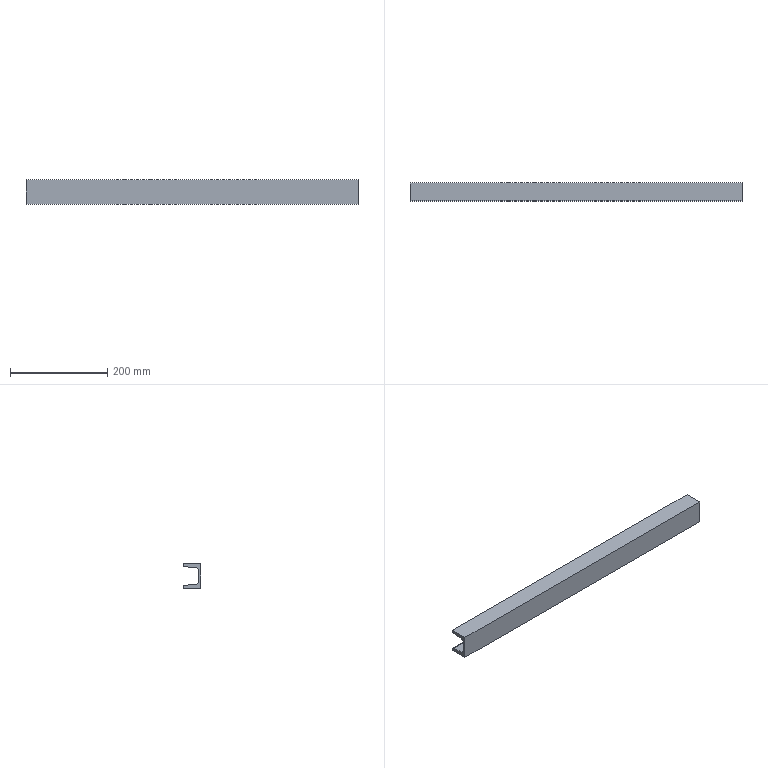Part | SolidWorks | features WeldMemberFeat 1, WeldmentFeature 1 | 1 solid | 14 faces | box 684 x 37 x 50 mm | volume 473534 mm3 | plane 10 | cylinder 4 | commonest cylinder face diameters 7 x2 14 x2
STEP:
#1=CARTESIAN_POINT('',(-342.,33.866,44.379));
#2=VERTEX_POINT('',#1);
#3=CARTESIAN_POINT('',(-342.,37.,47.859));
#4=VERTEX_POINT('',#3);
#5=CARTESIAN_POINT('',(-342.,33.5,47.859));
#6=DIRECTION('',(1.,0.,0.));
#7=DIRECTION('',(0.,1.,0.));
#8=AXIS2_PLACEMENT_3D('',#5,#6,#7);
#9=CIRCLE('',#8,3.5);
#10=EDGE_CURVE('',#2,#4,#9,.T.);
#11=ORIENTED_EDGE('',*,*,#10,.T.);
#12=CARTESIAN_POINT('',(342.,37.,47.859));
#13=VERTEX_POINT('',#12);
#14=CARTESIAN_POINT('',(342.,37.,47.859));
#15=DIRECTION('',(-1.,0.,0.));
#16=VECTOR('',#15,1000.);
#17=LINE('',#14,#16);
#18=EDGE_CURVE('',#13,#4,#17,.T.);
#19=ORIENTED_EDGE('',*,*,#18,.F.);
#20=CARTESIAN_POINT('',(342.,33.866,44.379));
#21=VERTEX_POINT('',#20);
#22=CARTESIAN_POINT('',(342.,33.5,47.859));
#23=DIRECTION('',(1.,0.,0.));
#24=DIRECTION('',(0.,1.,0.));
#25=AXIS2_PLACEMENT_3D('',#22,#23,#24);
#26=CIRCLE('',#25,3.5);
#27=EDGE_CURVE('',#21,#13,#26,.T.);
#28=ORIENTED_EDGE('',*,*,#27,.F.);
#29=CARTESIAN_POINT('',(342.,33.866,44.379));
#30=DIRECTION('',(-1.,0.,0.));
#31=VECTOR('',#30,1000.);
#32=LINE('',#29,#31);
#33=EDGE_CURVE('',#21,#2,#32,.T.);
#34=ORIENTED_EDGE('',*,*,#33,.T.);
#35=EDGE_LOOP('',(#11,#19,#28,#34));
#36=FACE_OUTER_BOUND('',#35,.T.);
#37=CARTESIAN_POINT('',(342.,33.5,47.859));
#38=DIRECTION('',(-1.,0.,0.));
#39=DIRECTION('',(0.,-1.,0.));
#40=AXIS2_PLACEMENT_3D('',#37,#38,#39);
#41=CYLINDRICAL_SURFACE('',#40,3.5);
#42=ADVANCED_FACE('',(#36),#41,.T.);
#43=CARTESIAN_POINT('',(-342.,37.,50.));
#44=VERTEX_POINT('',#43);
#45=CARTESIAN_POINT('',(-342.,37.,50.));
#46=DIRECTION('',(0.,0.,1.));
#47=VECTOR('',#46,1000.);
#48=LINE('',#45,#47);
#49=EDGE_CURVE('',#4,#44,#48,.T.);
#50=ORIENTED_EDGE('',*,*,#49,.T.);
#51=CARTESIAN_POINT('',(342.,37.,50.));
#52=VERTEX_POINT('',#51);
#53=CARTESIAN_POINT('',(342.,37.,50.));
#54=DIRECTION('',(-1.,0.,0.));
#55=VECTOR('',#54,1000.);
#56=LINE('',#53,#55);
#57=EDGE_CURVE('',#52,#44,#56,.T.);
#58=ORIENTED_EDGE('',*,*,#57,.F.);
#59=CARTESIAN_POINT('',(342.,37.,50.));
#60=DIRECTION('',(0.,0.,1.));
#61=VECTOR('',#60,1000.);
#62=LINE('',#59,#61);
#63=EDGE_CURVE('',#13,#52,#62,.T.);
#64=ORIENTED_EDGE('',*,*,#63,.F.);
#65=ORIENTED_EDGE('',*,*,#18,.T.);
#66=EDGE_LOOP('',(#50,#58,#64,#65));
#67=FACE_OUTER_BOUND('',#66,.T.);
#68=CARTESIAN_POINT('',(342.,37.,50.));
#69=DIRECTION('',(0.,-1.,0.));
#70=DIRECTION('',(1.,0.,0.));
#71=AXIS2_PLACEMENT_3D('',#68,#69,#70);
#72=PLANE('',#71);
#73=ADVANCED_FACE('',(#67),#72,.F.);
#74=CARTESIAN_POINT('',(-342.,0.,50.));
#75=VERTEX_POINT('',#74);
#76=CARTESIAN_POINT('',(-342.,37.,50.));
#77=DIRECTION('',(0.,-1.,0.));
#78=VECTOR('',#77,1000.);
#79=LINE('',#76,#78);
#80=EDGE_CURVE('',#44,#75,#79,.T.);
#81=ORIENTED_EDGE('',*,*,#80,.T.);
#82=CARTESIAN_POINT('',(342.,0.,50.));
#83=VERTEX_POINT('',#82);
#84=CARTESIAN_POINT('',(342.,0.,50.));
#85=DIRECTION('',(-1.,0.,0.));
#86=VECTOR('',#85,1000.);
#87=LINE('',#84,#86);
#88=EDGE_CURVE('',#83,#75,#87,.T.);
#89=ORIENTED_EDGE('',*,*,#88,.F.);
#90=CARTESIAN_POINT('',(342.,37.,50.));
#91=DIRECTION('',(0.,-1.,0.));
#92=VECTOR('',#91,1000.);
#93=LINE('',#90,#92);
#94=EDGE_CURVE('',#52,#83,#93,.T.);
#95=ORIENTED_EDGE('',*,*,#94,.F.);
#96=ORIENTED_EDGE('',*,*,#57,.T.);
#97=EDGE_LOOP('',(#81,#89,#95,#96));
#98=FACE_OUTER_BOUND('',#97,.T.);
#99=CARTESIAN_POINT('',(342.,37.,50.));
#100=DIRECTION('',(0.,0.,-1.));
#101=DIRECTION('',(0.,1.,0.));
#102=AXIS2_PLACEMENT_3D('',#99,#100,#101);
#103=PLANE('',#102);
#104=ADVANCED_FACE('',(#98),#103,.F.);
#105=CARTESIAN_POINT('',(-342.,0.,0.));
#106=VERTEX_POINT('',#105);
#107=CARTESIAN_POINT('',(-342.,0.,50.));
#108=DIRECTION('',(0.,0.,-1.));
#109=VECTOR('',#108,1000.);
#110=LINE('',#107,#109);
#111=EDGE_CURVE('',#75,#106,#110,.T.);
#112=ORIENTED_EDGE('',*,*,#111,.T.);
#113=CARTESIAN_POINT('',(342.,0.,0.));
#114=VERTEX_POINT('',#113);
#115=CARTESIAN_POINT('',(342.,0.,0.));
#116=DIRECTION('',(-1.,0.,0.));
#117=VECTOR('',#116,1000.);
#118=LINE('',#115,#117);
#119=EDGE_CURVE('',#114,#106,#118,.T.);
#120=ORIENTED_EDGE('',*,*,#119,.F.);
#121=CARTESIAN_POINT('',(342.,0.,50.));
#122=DIRECTION('',(0.,0.,-1.));
#123=VECTOR('',#122,1000.);
#124=LINE('',#121,#123);
#125=EDGE_CURVE('',#83,#114,#124,.T.);
#126=ORIENTED_EDGE('',*,*,#125,.F.);
#127=ORIENTED_EDGE('',*,*,#88,.T.);
#128=EDGE_LOOP('',(#112,#120,#126,#127));
#129=FACE_OUTER_BOUND('',#128,.T.);
#130=CARTESIAN_POINT('',(342.,0.,50.));
#131=DIRECTION('',(0.,1.,0.));
#132=DIRECTION('',(-1.,0.,0.));
#133=AXIS2_PLACEMENT_3D('',#130,#131,#132);
#134=PLANE('',#133);
#135=ADVANCED_FACE('',(#129),#134,.F.);
#136=CARTESIAN_POINT('',(-342.,37.,0.));
#137=VERTEX_POINT('',#136);
#138=CARTESIAN_POINT('',(-342.,37.,0.));
#139=DIRECTION('',(0.,1.,0.));
#140=VECTOR('',#139,1000.);
#141=LINE('',#138,#140);
#142=EDGE_CURVE('',#106,#137,#141,.T.);
#143=ORIENTED_EDGE('',*,*,#142,.T.);
#144=CARTESIAN_POINT('',(342.,37.,0.));
#145=VERTEX_POINT('',#144);
#146=CARTESIAN_POINT('',(342.,37.,0.));
#147=DIRECTION('',(-1.,0.,0.));
#148=VECTOR('',#147,1000.);
#149=LINE('',#146,#148);
#150=EDGE_CURVE('',#145,#137,#149,.T.);
#151=ORIENTED_EDGE('',*,*,#150,.F.);
#152=CARTESIAN_POINT('',(342.,37.,0.));
#153=DIRECTION('',(0.,1.,0.));
#154=VECTOR('',#153,1000.);
#155=LINE('',#152,#154);
#156=EDGE_CURVE('',#114,#145,#155,.T.);
#157=ORIENTED_EDGE('',*,*,#156,.F.);
#158=ORIENTED_EDGE('',*,*,#119,.T.);
#159=EDGE_LOOP('',(#143,#151,#157,#158));
#160=FACE_OUTER_BOUND('',#159,.T.);
#161=CARTESIAN_POINT('',(342.,37.,0.));
#162=DIRECTION('',(0.,0.,1.));
#163=DIRECTION('',(0.,-1.,0.));
#164=AXIS2_PLACEMENT_3D('',#161,#162,#163);
#165=PLANE('',#164);
#166=ADVANCED_FACE('',(#160),#165,.F.);
#167=CARTESIAN_POINT('',(-342.,37.,2.141));
#168=VERTEX_POINT('',#167);
#169=CARTESIAN_POINT('',(-342.,37.,0.));
#170=DIRECTION('',(0.,0.,1.));
#171=VECTOR('',#170,1000.);
#172=LINE('',#169,#171);
#173=EDGE_CURVE('',#137,#168,#172,.T.);
#174=ORIENTED_EDGE('',*,*,#173,.T.);
#175=CARTESIAN_POINT('',(342.,37.,2.141));
#176=VERTEX_POINT('',#175);
#177=CARTESIAN_POINT('',(342.,37.,2.141));
#178=DIRECTION('',(-1.,0.,0.));
#179=VECTOR('',#178,1000.);
#180=LINE('',#177,#179);
#181=EDGE_CURVE('',#176,#168,#180,.T.);
#182=ORIENTED_EDGE('',*,*,#181,.F.);
#183=CARTESIAN_POINT('',(342.,37.,0.));
#184=DIRECTION('',(0.,0.,1.));
#185=VECTOR('',#184,1000.);
#186=LINE('',#183,#185);
#187=EDGE_CURVE('',#145,#176,#186,.T.);
#188=ORIENTED_EDGE('',*,*,#187,.F.);
#189=ORIENTED_EDGE('',*,*,#150,.T.);
#190=EDGE_LOOP('',(#174,#182,#188,#189));
#191=FACE_OUTER_BOUND('',#190,.T.);
#192=CARTESIAN_POINT('',(342.,37.,0.));
#193=DIRECTION('',(0.,-1.,0.));
#194=DIRECTION('',(1.,0.,0.));
#195=AXIS2_PLACEMENT_3D('',#192,#193,#194);
#196=PLANE('',#195);
#197=ADVANCED_FACE('',(#191),#196,.F.);
#198=CARTESIAN_POINT('',(-342.,33.866,5.621));
#199=VERTEX_POINT('',#198);
#200=CARTESIAN_POINT('',(-342.,33.5,2.141));
#201=DIRECTION('',(1.,0.,0.));
#202=DIRECTION('',(0.,-1.,0.));
#203=AXIS2_PLACEMENT_3D('',#200,#201,#202);
#204=CIRCLE('',#203,3.5);
#205=EDGE_CURVE('',#168,#199,#204,.T.);
#206=ORIENTED_EDGE('',*,*,#205,.T.);
#207=CARTESIAN_POINT('',(342.,33.866,5.621));
#208=VERTEX_POINT('',#207);
#209=CARTESIAN_POINT('',(342.,33.866,5.621));
#210=DIRECTION('',(-1.,0.,0.));
#211=VECTOR('',#210,1000.);
#212=LINE('',#209,#211);
#213=EDGE_CURVE('',#208,#199,#212,.T.);
#214=ORIENTED_EDGE('',*,*,#213,.F.);
#215=CARTESIAN_POINT('',(342.,33.5,2.141));
#216=DIRECTION('',(1.,0.,0.));
#217=DIRECTION('',(0.,-1.,0.));
#218=AXIS2_PLACEMENT_3D('',#215,#216,#217);
#219=CIRCLE('',#218,3.5);
#220=EDGE_CURVE('',#176,#208,#219,.T.);
#221=ORIENTED_EDGE('',*,*,#220,.F.);
#222=ORIENTED_EDGE('',*,*,#181,.T.);
#223=EDGE_LOOP('',(#206,#214,#221,#222));
#224=FACE_OUTER_BOUND('',#223,.T.);
#225=CARTESIAN_POINT('',(342.,33.5,2.141));
#226=DIRECTION('',(-1.,0.,0.));
#227=DIRECTION('',(0.,-1.,0.));
#228=AXIS2_PLACEMENT_3D('',#225,#226,#227);
#229=CYLINDRICAL_SURFACE('',#228,3.5);
#230=ADVANCED_FACE('',(#224),#229,.T.);
#231=CARTESIAN_POINT('',(-342.,10.768,8.049));
#232=VERTEX_POINT('',#231);
#233=CARTESIAN_POINT('',(-342.,10.768,8.049));
#234=DIRECTION('',(0.,-0.9945,0.1045));
#235=VECTOR('',#234,1000.);
#236=LINE('',#233,#235);
#237=EDGE_CURVE('',#199,#232,#236,.T.);
#238=ORIENTED_EDGE('',*,*,#237,.T.);
#239=CARTESIAN_POINT('',(342.,10.768,8.049));
#240=VERTEX_POINT('',#239);
#241=CARTESIAN_POINT('',(342.,10.768,8.049));
#242=DIRECTION('',(-1.,0.,0.));
#243=VECTOR('',#242,1000.);
#244=LINE('',#241,#243);
#245=EDGE_CURVE('',#240,#232,#244,.T.);
#246=ORIENTED_EDGE('',*,*,#245,.F.);
#247=CARTESIAN_POINT('',(342.,10.768,8.049));
#248=DIRECTION('',(0.,-0.9945,0.1045));
#249=VECTOR('',#248,1000.);
#250=LINE('',#247,#249);
#251=EDGE_CURVE('',#208,#240,#250,.T.);
#252=ORIENTED_EDGE('',*,*,#251,.F.);
#253=ORIENTED_EDGE('',*,*,#213,.T.);
#254=EDGE_LOOP('',(#238,#246,#252,#253));
#255=FACE_OUTER_BOUND('',#254,.T.);
#256=CARTESIAN_POINT('',(342.,10.768,8.049));
#257=DIRECTION('',(0.,-0.1045,-0.9945));
#258=DIRECTION('',(0.,0.9945,-0.1045));
#259=AXIS2_PLACEMENT_3D('',#256,#257,#258);
#260=PLANE('',#259);
#261=ADVANCED_FACE('',(#255),#260,.F.);
#262=CARTESIAN_POINT('',(-342.,4.5,15.011));
#263=VERTEX_POINT('',#262);
#264=CARTESIAN_POINT('',(-342.,11.5,15.011));
#265=DIRECTION('',(-1.,0.,0.));
#266=DIRECTION('',(0.,1.,0.));
#267=AXIS2_PLACEMENT_3D('',#264,#265,#266);
#268=CIRCLE('',#267,7.);
#269=EDGE_CURVE('',#232,#263,#268,.T.);
#270=ORIENTED_EDGE('',*,*,#269,.T.);
#271=CARTESIAN_POINT('',(342.,4.5,15.011));
#272=VERTEX_POINT('',#271);
#273=CARTESIAN_POINT('',(342.,4.5,15.011));
#274=DIRECTION('',(-1.,0.,0.));
#275=VECTOR('',#274,1000.);
#276=LINE('',#273,#275);
#277=EDGE_CURVE('',#272,#263,#276,.T.);
#278=ORIENTED_EDGE('',*,*,#277,.F.);
#279=CARTESIAN_POINT('',(342.,11.5,15.011));
#280=DIRECTION('',(-1.,0.,0.));
#281=DIRECTION('',(0.,1.,0.));
#282=AXIS2_PLACEMENT_3D('',#279,#280,#281);
#283=CIRCLE('',#282,7.);
#284=EDGE_CURVE('',#240,#272,#283,.T.);
#285=ORIENTED_EDGE('',*,*,#284,.F.);
#286=ORIENTED_EDGE('',*,*,#245,.T.);
#287=EDGE_LOOP('',(#270,#278,#285,#286));
#288=FACE_OUTER_BOUND('',#287,.T.);
#289=CARTESIAN_POINT('',(342.,11.5,15.011));
#290=DIRECTION('',(-1.,0.,0.));
#291=DIRECTION('',(0.,-1.,0.));
#292=AXIS2_PLACEMENT_3D('',#289,#290,#291);
#293=CYLINDRICAL_SURFACE('',#292,7.);
#294=ADVANCED_FACE('',(#288),#293,.F.);
#295=CARTESIAN_POINT('',(-342.,4.5,34.989));
#296=VERTEX_POINT('',#295);
#297=CARTESIAN_POINT('',(-342.,4.5,34.989));
#298=DIRECTION('',(0.,0.,1.));
#299=VECTOR('',#298,1000.);
#300=LINE('',#297,#299);
#301=EDGE_CURVE('',#263,#296,#300,.T.);
#302=ORIENTED_EDGE('',*,*,#301,.T.);
#303=CARTESIAN_POINT('',(342.,4.5,34.989));
#304=VERTEX_POINT('',#303);
#305=CARTESIAN_POINT('',(342.,4.5,34.989));
#306=DIRECTION('',(-1.,0.,0.));
#307=VECTOR('',#306,1000.);
#308=LINE('',#305,#307);
#309=EDGE_CURVE('',#304,#296,#308,.T.);
#310=ORIENTED_EDGE('',*,*,#309,.F.);
#311=CARTESIAN_POINT('',(342.,4.5,34.989));
#312=DIRECTION('',(0.,0.,1.));
#313=VECTOR('',#312,1000.);
#314=LINE('',#311,#313);
#315=EDGE_CURVE('',#272,#304,#314,.T.);
#316=ORIENTED_EDGE('',*,*,#315,.F.);
#317=ORIENTED_EDGE('',*,*,#277,.T.);
#318=EDGE_LOOP('',(#302,#310,#316,#317));
#319=FACE_OUTER_BOUND('',#318,.T.);
#320=CARTESIAN_POINT('',(342.,4.5,34.989));
#321=DIRECTION('',(0.,-1.,0.));
#322=DIRECTION('',(1.,0.,0.));
#323=AXIS2_PLACEMENT_3D('',#320,#321,#322);
#324=PLANE('',#323);
#325=ADVANCED_FACE('',(#319),#324,.F.);
#326=CARTESIAN_POINT('',(-342.,10.768,41.951));
#327=VERTEX_POINT('',#326);
#328=CARTESIAN_POINT('',(-342.,11.5,34.989));
#329=DIRECTION('',(-1.,0.,0.));
#330=DIRECTION('',(0.,-1.,0.));
#331=AXIS2_PLACEMENT_3D('',#328,#329,#330);
#332=CIRCLE('',#331,7.);
#333=EDGE_CURVE('',#296,#327,#332,.T.);
#334=ORIENTED_EDGE('',*,*,#333,.T.);
#335=CARTESIAN_POINT('',(342.,10.768,41.951));
#336=VERTEX_POINT('',#335);
#337=CARTESIAN_POINT('',(342.,10.768,41.951));
#338=DIRECTION('',(-1.,0.,0.));
#339=VECTOR('',#338,1000.);
#340=LINE('',#337,#339);
#341=EDGE_CURVE('',#336,#327,#340,.T.);
#342=ORIENTED_EDGE('',*,*,#341,.F.);
#343=CARTESIAN_POINT('',(342.,11.5,34.989));
#344=DIRECTION('',(-1.,0.,0.));
#345=DIRECTION('',(0.,-1.,0.));
#346=AXIS2_PLACEMENT_3D('',#343,#344,#345);
#347=CIRCLE('',#346,7.);
#348=EDGE_CURVE('',#304,#336,#347,.T.);
#349=ORIENTED_EDGE('',*,*,#348,.F.);
#350=ORIENTED_EDGE('',*,*,#309,.T.);
#351=EDGE_LOOP('',(#334,#342,#349,#350));
#352=FACE_OUTER_BOUND('',#351,.T.);
#353=CARTESIAN_POINT('',(342.,11.5,34.989));
#354=DIRECTION('',(-1.,0.,0.));
#355=DIRECTION('',(0.,-1.,0.));
#356=AXIS2_PLACEMENT_3D('',#353,#354,#355);
#357=CYLINDRICAL_SURFACE('',#356,7.);
#358=ADVANCED_FACE('',(#352),#357,.F.);
#359=CARTESIAN_POINT('',(-342.,10.768,41.951));
#360=DIRECTION('',(0.,0.9945,0.1045));
#361=VECTOR('',#360,1000.);
#362=LINE('',#359,#361);
#363=EDGE_CURVE('',#327,#2,#362,.T.);
#364=ORIENTED_EDGE('',*,*,#363,.T.);
#365=ORIENTED_EDGE('',*,*,#33,.F.);
#366=CARTESIAN_POINT('',(342.,10.768,41.951));
#367=DIRECTION('',(0.,0.9945,0.1045));
#368=VECTOR('',#367,1000.);
#369=LINE('',#366,#368);
#370=EDGE_CURVE('',#336,#21,#369,.T.);
#371=ORIENTED_EDGE('',*,*,#370,.F.);
#372=ORIENTED_EDGE('',*,*,#341,.T.);
#373=EDGE_LOOP('',(#364,#365,#371,#372));
#374=FACE_OUTER_BOUND('',#373,.T.);
#375=CARTESIAN_POINT('',(342.,10.768,41.951));
#376=DIRECTION('',(0.,-0.1045,0.9945));
#377=DIRECTION('',(0.,-0.9945,-0.1045));
#378=AXIS2_PLACEMENT_3D('',#375,#376,#377);
#379=PLANE('',#378);
#380=ADVANCED_FACE('',(#374),#379,.F.);
#381=ORIENTED_EDGE('',*,*,#27,.T.);
#382=ORIENTED_EDGE('',*,*,#63,.T.);
#383=ORIENTED_EDGE('',*,*,#94,.T.);
#384=ORIENTED_EDGE('',*,*,#125,.T.);
#385=ORIENTED_EDGE('',*,*,#156,.T.);
#386=ORIENTED_EDGE('',*,*,#187,.T.);
#387=ORIENTED_EDGE('',*,*,#220,.T.);
#388=ORIENTED_EDGE('',*,*,#251,.T.);
#389=ORIENTED_EDGE('',*,*,#284,.T.);
#390=ORIENTED_EDGE('',*,*,#315,.T.);
#391=ORIENTED_EDGE('',*,*,#348,.T.);
#392=ORIENTED_EDGE('',*,*,#370,.T.);
#393=EDGE_LOOP('',(#381,#382,#383,#384,#385,#386,#387,#388,#389,#390,#391,#392));
#394=FACE_OUTER_BOUND('',#393,.T.);
#395=CARTESIAN_POINT('',(342.,33.5,47.859));
#396=DIRECTION('',(1.,0.,0.));
#397=DIRECTION('',(0.,1.,0.));
#398=AXIS2_PLACEMENT_3D('',#395,#396,#397);
#399=PLANE('',#398);
#400=ADVANCED_FACE('',(#394),#399,.T.);
#401=ORIENTED_EDGE('',*,*,#10,.F.);
#402=ORIENTED_EDGE('',*,*,#363,.F.);
#403=ORIENTED_EDGE('',*,*,#333,.F.);
#404=ORIENTED_EDGE('',*,*,#301,.F.);
#405=ORIENTED_EDGE('',*,*,#269,.F.);
#406=ORIENTED_EDGE('',*,*,#237,.F.);
#407=ORIENTED_EDGE('',*,*,#205,.F.);
#408=ORIENTED_EDGE('',*,*,#173,.F.);
#409=ORIENTED_EDGE('',*,*,#142,.F.);
#410=ORIENTED_EDGE('',*,*,#111,.F.);
#411=ORIENTED_EDGE('',*,*,#80,.F.);
#412=ORIENTED_EDGE('',*,*,#49,.F.);
#413=EDGE_LOOP('',(#401,#402,#403,#404,#405,#406,#407,#408,#409,#410,#411,#412));
#414=FACE_OUTER_BOUND('',#413,.T.);
#415=CARTESIAN_POINT('',(-342.,33.5,47.859));
#416=DIRECTION('',(1.,0.,0.));
#417=DIRECTION('',(0.,1.,0.));
#418=AXIS2_PLACEMENT_3D('',#415,#416,#417);
#419=PLANE('',#418);
#420=ADVANCED_FACE('',(#414),#419,.F.);
#421=CLOSED_SHELL('',(#42,#73,#104,#135,#166,#197,#230,#261,#294,#325,#358,#380,#400,#420));
#422=MANIFOLD_SOLID_BREP('',#421);
#423=CARTESIAN_POINT('',(0.,0.,0.));
#424=DIRECTION('',(0.,0.,1.));
#425=DIRECTION('',(1.,0.,0.));
#426=AXIS2_PLACEMENT_3D('',#423,#424,#425);
#427=(LENGTH_UNIT()NAMED_UNIT(*)SI_UNIT(.MILLI.,.METRE.));
#428=UNCERTAINTY_MEASURE_WITH_UNIT(LENGTH_MEASURE(0.00001),#427,'','');
#429=(NAMED_UNIT(*)PLANE_ANGLE_UNIT()SI_UNIT($,.RADIAN.));
#430=(NAMED_UNIT(*)SI_UNIT($,.STERADIAN.)SOLID_ANGLE_UNIT());
#431=(GEOMETRIC_REPRESENTATION_CONTEXT(3)GLOBAL_UNCERTAINTY_ASSIGNED_CONTEXT((#428))GLOBAL_UNIT_ASSIGNED_CONTEXT((#427,#429,#430))REPRESENTATION_CONTEXT('',''));
#432=ADVANCED_BREP_SHAPE_REPRESENTATION('',(#422,#426),#431);